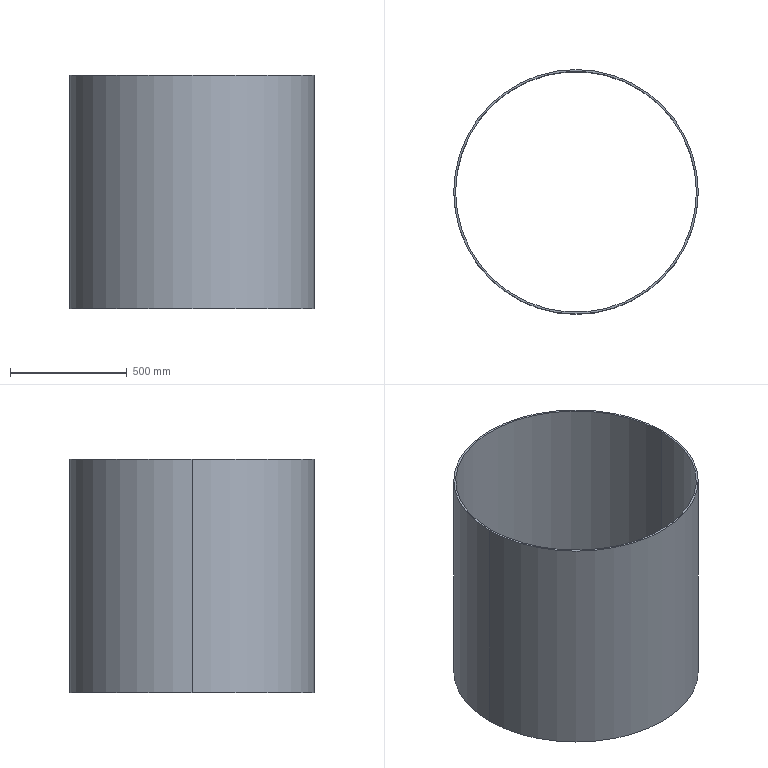Part | SolidWorks | features ExtruThin 1 | 1 solid | 6 faces | box 1046 x 1046 x 1000 mm | volume 26087785 mm3 | cylinder 4 | plane 2 | commonest cylinder face diameters 1030 x2 1046 x2
STEP:
#1=CARTESIAN_POINT('',(-515.,0.,500.));
#2=VERTEX_POINT('',#1);
#3=CARTESIAN_POINT('',(515.,0.,500.));
#4=VERTEX_POINT('',#3);
#5=CARTESIAN_POINT('',(0.,0.,500.));
#6=DIRECTION('',(0.,0.,1.));
#7=DIRECTION('',(1.,0.,0.));
#8=AXIS2_PLACEMENT_3D('',#5,#6,#7);
#9=CIRCLE('',#8,515.);
#10=EDGE_CURVE('',#2,#4,#9,.T.);
#11=ORIENTED_EDGE('',*,*,#10,.T.);
#12=CARTESIAN_POINT('',(515.,0.,-500.));
#13=VERTEX_POINT('',#12);
#14=CARTESIAN_POINT('',(515.,0.,500.));
#15=DIRECTION('',(0.,0.,-1.));
#16=VECTOR('',#15,1000.);
#17=LINE('',#14,#16);
#18=EDGE_CURVE('',#4,#13,#17,.T.);
#19=ORIENTED_EDGE('',*,*,#18,.T.);
#20=CARTESIAN_POINT('',(-515.,0.,-500.));
#21=VERTEX_POINT('',#20);
#22=CARTESIAN_POINT('',(0.,0.,-500.));
#23=DIRECTION('',(0.,0.,1.));
#24=DIRECTION('',(1.,0.,0.));
#25=AXIS2_PLACEMENT_3D('',#22,#23,#24);
#26=CIRCLE('',#25,515.);
#27=EDGE_CURVE('',#21,#13,#26,.T.);
#28=ORIENTED_EDGE('',*,*,#27,.F.);
#29=CARTESIAN_POINT('',(-515.,0.,500.));
#30=DIRECTION('',(0.,0.,-1.));
#31=VECTOR('',#30,1000.);
#32=LINE('',#29,#31);
#33=EDGE_CURVE('',#2,#21,#32,.T.);
#34=ORIENTED_EDGE('',*,*,#33,.F.);
#35=EDGE_LOOP('',(#11,#19,#28,#34));
#36=FACE_OUTER_BOUND('',#35,.T.);
#37=CARTESIAN_POINT('',(0.,0.,500.));
#38=DIRECTION('',(0.,0.,-1.));
#39=DIRECTION('',(-1.,0.,0.));
#40=AXIS2_PLACEMENT_3D('',#37,#38,#39);
#41=CYLINDRICAL_SURFACE('',#40,515.);
#42=ADVANCED_FACE('',(#36),#41,.F.);
#43=CARTESIAN_POINT('',(523.,0.,500.));
#44=VERTEX_POINT('',#43);
#45=CARTESIAN_POINT('',(-523.,0.,500.));
#46=VERTEX_POINT('',#45);
#47=CARTESIAN_POINT('',(0.,0.,500.));
#48=DIRECTION('',(0.,0.,1.));
#49=DIRECTION('',(1.,0.,0.));
#50=AXIS2_PLACEMENT_3D('',#47,#48,#49);
#51=CIRCLE('',#50,523.);
#52=EDGE_CURVE('',#44,#46,#51,.T.);
#53=ORIENTED_EDGE('',*,*,#52,.F.);
#54=CARTESIAN_POINT('',(523.,0.,-500.));
#55=VERTEX_POINT('',#54);
#56=CARTESIAN_POINT('',(523.,0.,500.));
#57=DIRECTION('',(0.,0.,-1.));
#58=VECTOR('',#57,1000.);
#59=LINE('',#56,#58);
#60=EDGE_CURVE('',#44,#55,#59,.T.);
#61=ORIENTED_EDGE('',*,*,#60,.T.);
#62=CARTESIAN_POINT('',(-523.,0.,-500.));
#63=VERTEX_POINT('',#62);
#64=CARTESIAN_POINT('',(0.,0.,-500.));
#65=DIRECTION('',(0.,0.,1.));
#66=DIRECTION('',(1.,0.,0.));
#67=AXIS2_PLACEMENT_3D('',#64,#65,#66);
#68=CIRCLE('',#67,523.);
#69=EDGE_CURVE('',#55,#63,#68,.T.);
#70=ORIENTED_EDGE('',*,*,#69,.T.);
#71=CARTESIAN_POINT('',(-523.,0.,500.));
#72=DIRECTION('',(0.,0.,-1.));
#73=VECTOR('',#72,1000.);
#74=LINE('',#71,#73);
#75=EDGE_CURVE('',#46,#63,#74,.T.);
#76=ORIENTED_EDGE('',*,*,#75,.F.);
#77=EDGE_LOOP('',(#53,#61,#70,#76));
#78=FACE_OUTER_BOUND('',#77,.T.);
#79=CARTESIAN_POINT('',(0.,0.,500.));
#80=DIRECTION('',(0.,0.,-1.));
#81=DIRECTION('',(-1.,0.,0.));
#82=AXIS2_PLACEMENT_3D('',#79,#80,#81);
#83=CYLINDRICAL_SURFACE('',#82,523.);
#84=ADVANCED_FACE('',(#78),#83,.T.);
#85=CARTESIAN_POINT('',(0.,0.,500.));
#86=DIRECTION('',(0.,0.,1.));
#87=DIRECTION('',(1.,0.,0.));
#88=AXIS2_PLACEMENT_3D('',#85,#86,#87);
#89=CIRCLE('',#88,523.);
#90=EDGE_CURVE('',#46,#44,#89,.T.);
#91=ORIENTED_EDGE('',*,*,#90,.T.);
#92=ORIENTED_EDGE('',*,*,#52,.T.);
#93=EDGE_LOOP('',(#91,#92));
#94=FACE_OUTER_BOUND('',#93,.T.);
#95=ORIENTED_EDGE('',*,*,#10,.F.);
#96=CARTESIAN_POINT('',(0.,0.,500.));
#97=DIRECTION('',(0.,0.,1.));
#98=DIRECTION('',(1.,0.,0.));
#99=AXIS2_PLACEMENT_3D('',#96,#97,#98);
#100=CIRCLE('',#99,515.);
#101=EDGE_CURVE('',#4,#2,#100,.T.);
#102=ORIENTED_EDGE('',*,*,#101,.F.);
#103=EDGE_LOOP('',(#95,#102));
#104=FACE_BOUND('',#103,.T.);
#105=CARTESIAN_POINT('',(0.,0.,500.));
#106=DIRECTION('',(0.,0.,1.));
#107=DIRECTION('',(1.,0.,0.));
#108=AXIS2_PLACEMENT_3D('',#105,#106,#107);
#109=PLANE('',#108);
#110=ADVANCED_FACE('',(#94,#104),#109,.T.);
#111=CARTESIAN_POINT('',(0.,0.,-500.));
#112=DIRECTION('',(0.,0.,1.));
#113=DIRECTION('',(1.,0.,0.));
#114=AXIS2_PLACEMENT_3D('',#111,#112,#113);
#115=CIRCLE('',#114,523.);
#116=EDGE_CURVE('',#63,#55,#115,.T.);
#117=ORIENTED_EDGE('',*,*,#116,.F.);
#118=ORIENTED_EDGE('',*,*,#69,.F.);
#119=EDGE_LOOP('',(#117,#118));
#120=FACE_OUTER_BOUND('',#119,.T.);
#121=ORIENTED_EDGE('',*,*,#27,.T.);
#122=CARTESIAN_POINT('',(0.,0.,-500.));
#123=DIRECTION('',(0.,0.,1.));
#124=DIRECTION('',(1.,0.,0.));
#125=AXIS2_PLACEMENT_3D('',#122,#123,#124);
#126=CIRCLE('',#125,515.);
#127=EDGE_CURVE('',#13,#21,#126,.T.);
#128=ORIENTED_EDGE('',*,*,#127,.T.);
#129=EDGE_LOOP('',(#121,#128));
#130=FACE_BOUND('',#129,.T.);
#131=CARTESIAN_POINT('',(0.,0.,-500.));
#132=DIRECTION('',(0.,0.,1.));
#133=DIRECTION('',(1.,0.,0.));
#134=AXIS2_PLACEMENT_3D('',#131,#132,#133);
#135=PLANE('',#134);
#136=ADVANCED_FACE('',(#120,#130),#135,.F.);
#137=ORIENTED_EDGE('',*,*,#60,.F.);
#138=ORIENTED_EDGE('',*,*,#90,.F.);
#139=ORIENTED_EDGE('',*,*,#75,.T.);
#140=ORIENTED_EDGE('',*,*,#116,.T.);
#141=EDGE_LOOP('',(#137,#138,#139,#140));
#142=FACE_OUTER_BOUND('',#141,.T.);
#143=CARTESIAN_POINT('',(0.,0.,500.));
#144=DIRECTION('',(0.,0.,-1.));
#145=DIRECTION('',(-1.,0.,0.));
#146=AXIS2_PLACEMENT_3D('',#143,#144,#145);
#147=CYLINDRICAL_SURFACE('',#146,523.);
#148=ADVANCED_FACE('',(#142),#147,.T.);
#149=ORIENTED_EDGE('',*,*,#18,.F.);
#150=ORIENTED_EDGE('',*,*,#101,.T.);
#151=ORIENTED_EDGE('',*,*,#33,.T.);
#152=ORIENTED_EDGE('',*,*,#127,.F.);
#153=EDGE_LOOP('',(#149,#150,#151,#152));
#154=FACE_OUTER_BOUND('',#153,.T.);
#155=CARTESIAN_POINT('',(0.,0.,500.));
#156=DIRECTION('',(0.,0.,-1.));
#157=DIRECTION('',(-1.,0.,0.));
#158=AXIS2_PLACEMENT_3D('',#155,#156,#157);
#159=CYLINDRICAL_SURFACE('',#158,515.);
#160=ADVANCED_FACE('',(#154),#159,.F.);
#161=CLOSED_SHELL('',(#42,#84,#110,#136,#148,#160));
#162=MANIFOLD_SOLID_BREP('',#161);
#163=CARTESIAN_POINT('',(0.,0.,0.));
#164=DIRECTION('',(0.,0.,1.));
#165=DIRECTION('',(1.,0.,0.));
#166=AXIS2_PLACEMENT_3D('',#163,#164,#165);
#167=(LENGTH_UNIT()NAMED_UNIT(*)SI_UNIT(.MILLI.,.METRE.));
#168=UNCERTAINTY_MEASURE_WITH_UNIT(LENGTH_MEASURE(0.00001),#167,'','');
#169=(NAMED_UNIT(*)PLANE_ANGLE_UNIT()SI_UNIT($,.RADIAN.));
#170=(NAMED_UNIT(*)SI_UNIT($,.STERADIAN.)SOLID_ANGLE_UNIT());
#171=(GEOMETRIC_REPRESENTATION_CONTEXT(3)GLOBAL_UNCERTAINTY_ASSIGNED_CONTEXT((#168))GLOBAL_UNIT_ASSIGNED_CONTEXT((#167,#169,#170))REPRESENTATION_CONTEXT('',''));
#172=ADVANCED_BREP_SHAPE_REPRESENTATION('',(#162,#166),#171);